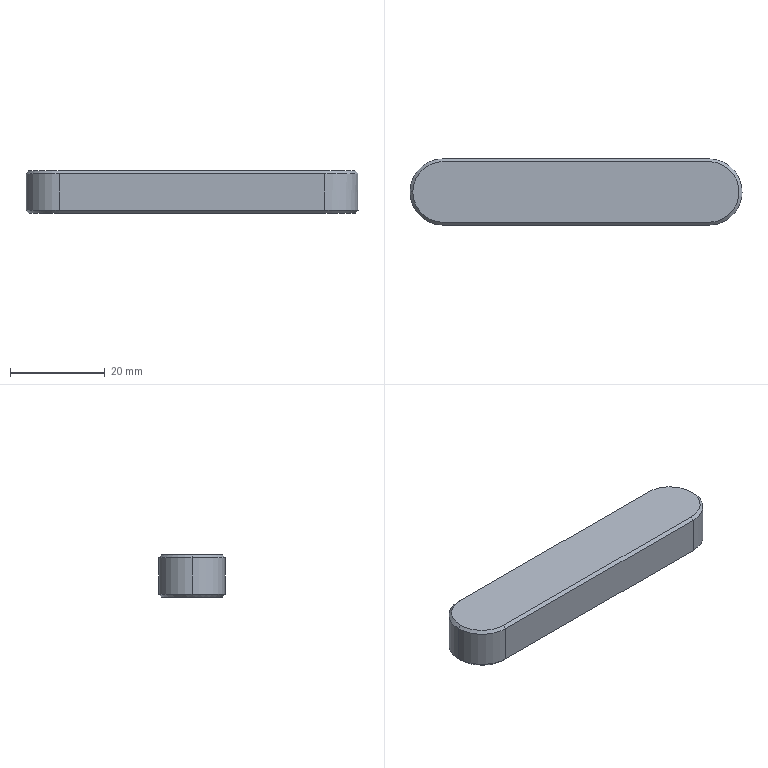Part | SolidWorks | features Boss 2, Chamfer 1, Extrusion 1 | 1 solid | 17 faces | box 70 x 14 x 9 mm | volume 8386 mm3 | plane 8 | cone 6 | cylinder 3 | commonest cylinder face diameters 14 x3
STEP:
#1=CARTESIAN_POINT('',(-62.4,0.,4.5));
#2=VERTEX_POINT('',#1);
#3=CARTESIAN_POINT('',(-56.,-6.4,4.5));
#4=VERTEX_POINT('',#3);
#5=CARTESIAN_POINT('',(-56.,0.,4.5));
#6=DIRECTION('',(0.,0.,1.));
#7=DIRECTION('',(-1.,0.,0.));
#8=AXIS2_PLACEMENT_3D('',#5,#6,#7);
#9=CIRCLE('',#8,6.4);
#10=EDGE_CURVE('',#2,#4,#9,.T.);
#11=ORIENTED_EDGE('',*,*,#10,.F.);
#12=CARTESIAN_POINT('',(-63.,0.,3.9));
#13=VERTEX_POINT('',#12);
#14=CARTESIAN_POINT('',(-62.4,0.,4.5));
#15=DIRECTION('',(-0.7071,0.,-0.7071));
#16=VECTOR('',#15,1000.);
#17=LINE('',#14,#16);
#18=EDGE_CURVE('',#2,#13,#17,.T.);
#19=ORIENTED_EDGE('',*,*,#18,.T.);
#20=CARTESIAN_POINT('',(-56.,-7.,3.9));
#21=VERTEX_POINT('',#20);
#22=CARTESIAN_POINT('',(-56.,0.,3.9));
#23=DIRECTION('',(0.,0.,-1.));
#24=DIRECTION('',(-1.,0.,0.));
#25=AXIS2_PLACEMENT_3D('',#22,#23,#24);
#26=CIRCLE('',#25,7.);
#27=EDGE_CURVE('',#21,#13,#26,.T.);
#28=ORIENTED_EDGE('',*,*,#27,.F.);
#29=CARTESIAN_POINT('',(-56.,-6.4,4.5));
#30=DIRECTION('',(0.,-0.7071,-0.7071));
#31=VECTOR('',#30,1000.);
#32=LINE('',#29,#31);
#33=EDGE_CURVE('',#4,#21,#32,.T.);
#34=ORIENTED_EDGE('',*,*,#33,.F.);
#35=EDGE_LOOP('',(#11,#19,#28,#34));
#36=FACE_OUTER_BOUND('',#35,.T.);
#37=CARTESIAN_POINT('',(-56.,0.,4.5));
#38=DIRECTION('',(0.,0.,-1.));
#39=DIRECTION('',(-1.,0.,0.));
#40=AXIS2_PLACEMENT_3D('',#37,#38,#39);
#41=CONICAL_SURFACE('',#40,6.4,0.7854);
#42=ADVANCED_FACE('',(#36),#41,.T.);
#43=CARTESIAN_POINT('',(6.4,0.,-4.5));
#44=VERTEX_POINT('',#43);
#45=CARTESIAN_POINT('',(0.,-6.4,-4.5));
#46=VERTEX_POINT('',#45);
#47=CARTESIAN_POINT('',(0.,0.,-4.5));
#48=DIRECTION('',(0.,0.,-1.));
#49=DIRECTION('',(-1.,0.,0.));
#50=AXIS2_PLACEMENT_3D('',#47,#48,#49);
#51=CIRCLE('',#50,6.4);
#52=EDGE_CURVE('',#44,#46,#51,.T.);
#53=ORIENTED_EDGE('',*,*,#52,.F.);
#54=CARTESIAN_POINT('',(7.,0.,-3.9));
#55=VERTEX_POINT('',#54);
#56=CARTESIAN_POINT('',(7.,0.,-3.9));
#57=DIRECTION('',(0.7071,0.,0.7071));
#58=VECTOR('',#57,1000.);
#59=LINE('',#56,#58);
#60=EDGE_CURVE('',#44,#55,#59,.T.);
#61=ORIENTED_EDGE('',*,*,#60,.T.);
#62=CARTESIAN_POINT('',(0.,-7.,-3.9));
#63=VERTEX_POINT('',#62);
#64=CARTESIAN_POINT('',(0.,0.,-3.9));
#65=DIRECTION('',(0.,0.,1.));
#66=DIRECTION('',(-1.,0.,0.));
#67=AXIS2_PLACEMENT_3D('',#64,#65,#66);
#68=CIRCLE('',#67,7.);
#69=EDGE_CURVE('',#63,#55,#68,.T.);
#70=ORIENTED_EDGE('',*,*,#69,.F.);
#71=CARTESIAN_POINT('',(0.,-6.4,-4.5));
#72=DIRECTION('',(0.,-0.7071,0.7071));
#73=VECTOR('',#72,1000.);
#74=LINE('',#71,#73);
#75=EDGE_CURVE('',#46,#63,#74,.T.);
#76=ORIENTED_EDGE('',*,*,#75,.F.);
#77=EDGE_LOOP('',(#53,#61,#70,#76));
#78=FACE_OUTER_BOUND('',#77,.T.);
#79=CARTESIAN_POINT('',(0.,0.,-3.9));
#80=DIRECTION('',(0.,0.,1.));
#81=DIRECTION('',(1.,0.,0.));
#82=AXIS2_PLACEMENT_3D('',#79,#80,#81);
#83=CONICAL_SURFACE('',#82,7.,0.7854);
#84=ADVANCED_FACE('',(#78),#83,.T.);
#85=ORIENTED_EDGE('',*,*,#27,.T.);
#86=CARTESIAN_POINT('',(-63.,0.,-3.9));
#87=VERTEX_POINT('',#86);
#88=CARTESIAN_POINT('',(-63.,0.,4.5));
#89=DIRECTION('',(0.,0.,-1.));
#90=VECTOR('',#89,1000.);
#91=LINE('',#88,#90);
#92=EDGE_CURVE('',#13,#87,#91,.T.);
#93=ORIENTED_EDGE('',*,*,#92,.T.);
#94=CARTESIAN_POINT('',(-56.,-7.,-3.9));
#95=VERTEX_POINT('',#94);
#96=CARTESIAN_POINT('',(-56.,0.,-3.9));
#97=DIRECTION('',(0.,0.,1.));
#98=DIRECTION('',(-1.,0.,0.));
#99=AXIS2_PLACEMENT_3D('',#96,#97,#98);
#100=CIRCLE('',#99,7.);
#101=EDGE_CURVE('',#87,#95,#100,.T.);
#102=ORIENTED_EDGE('',*,*,#101,.T.);
#103=CARTESIAN_POINT('',(-56.,-7.,4.5));
#104=DIRECTION('',(0.,0.,-1.));
#105=VECTOR('',#104,1000.);
#106=LINE('',#103,#105);
#107=EDGE_CURVE('',#21,#95,#106,.T.);
#108=ORIENTED_EDGE('',*,*,#107,.F.);
#109=EDGE_LOOP('',(#85,#93,#102,#108));
#110=FACE_OUTER_BOUND('',#109,.T.);
#111=CARTESIAN_POINT('',(-56.,0.,4.5));
#112=DIRECTION('',(0.,0.,-1.));
#113=DIRECTION('',(-1.,0.,0.));
#114=AXIS2_PLACEMENT_3D('',#111,#112,#113);
#115=CYLINDRICAL_SURFACE('',#114,7.);
#116=ADVANCED_FACE('',(#110),#115,.T.);
#117=ORIENTED_EDGE('',*,*,#92,.F.);
#118=CARTESIAN_POINT('',(-56.,7.,3.9));
#119=VERTEX_POINT('',#118);
#120=CARTESIAN_POINT('',(-56.,0.,3.9));
#121=DIRECTION('',(0.,0.,-1.));
#122=DIRECTION('',(-1.,0.,0.));
#123=AXIS2_PLACEMENT_3D('',#120,#121,#122);
#124=CIRCLE('',#123,7.);
#125=EDGE_CURVE('',#13,#119,#124,.T.);
#126=ORIENTED_EDGE('',*,*,#125,.T.);
#127=CARTESIAN_POINT('',(-56.,7.,-3.9));
#128=VERTEX_POINT('',#127);
#129=CARTESIAN_POINT('',(-56.,7.,4.5));
#130=DIRECTION('',(0.,0.,-1.));
#131=VECTOR('',#130,1000.);
#132=LINE('',#129,#131);
#133=EDGE_CURVE('',#119,#128,#132,.T.);
#134=ORIENTED_EDGE('',*,*,#133,.T.);
#135=CARTESIAN_POINT('',(-56.,0.,-3.9));
#136=DIRECTION('',(0.,0.,1.));
#137=DIRECTION('',(-1.,0.,0.));
#138=AXIS2_PLACEMENT_3D('',#135,#136,#137);
#139=CIRCLE('',#138,7.);
#140=EDGE_CURVE('',#128,#87,#139,.T.);
#141=ORIENTED_EDGE('',*,*,#140,.T.);
#142=EDGE_LOOP('',(#117,#126,#134,#141));
#143=FACE_OUTER_BOUND('',#142,.T.);
#144=CARTESIAN_POINT('',(-56.,0.,4.5));
#145=DIRECTION('',(0.,0.,-1.));
#146=DIRECTION('',(-1.,0.,0.));
#147=AXIS2_PLACEMENT_3D('',#144,#145,#146);
#148=CYLINDRICAL_SURFACE('',#147,7.);
#149=ADVANCED_FACE('',(#143),#148,.T.);
#150=ORIENTED_EDGE('',*,*,#107,.T.);
#151=CARTESIAN_POINT('',(0.,-7.,-3.9));
#152=DIRECTION('',(1.,0.,0.));
#153=VECTOR('',#152,1000.);
#154=LINE('',#151,#153);
#155=EDGE_CURVE('',#95,#63,#154,.T.);
#156=ORIENTED_EDGE('',*,*,#155,.T.);
#157=CARTESIAN_POINT('',(0.,-7.,3.9));
#158=VERTEX_POINT('',#157);
#159=CARTESIAN_POINT('',(0.,-7.,4.5));
#160=DIRECTION('',(0.,0.,-1.));
#161=VECTOR('',#160,1000.);
#162=LINE('',#159,#161);
#163=EDGE_CURVE('',#158,#63,#162,.T.);
#164=ORIENTED_EDGE('',*,*,#163,.F.);
#165=CARTESIAN_POINT('',(0.,-7.,3.9));
#166=DIRECTION('',(-1.,0.,0.));
#167=VECTOR('',#166,1000.);
#168=LINE('',#165,#167);
#169=EDGE_CURVE('',#158,#21,#168,.T.);
#170=ORIENTED_EDGE('',*,*,#169,.T.);
#171=EDGE_LOOP('',(#150,#156,#164,#170));
#172=FACE_OUTER_BOUND('',#171,.T.);
#173=CARTESIAN_POINT('',(0.,-7.,4.5));
#174=DIRECTION('',(0.,1.,0.));
#175=DIRECTION('',(-1.,0.,0.));
#176=AXIS2_PLACEMENT_3D('',#173,#174,#175);
#177=PLANE('',#176);
#178=ADVANCED_FACE('',(#172),#177,.F.);
#179=CARTESIAN_POINT('',(0.,7.,3.9));
#180=VERTEX_POINT('',#179);
#181=CARTESIAN_POINT('',(0.,7.,-3.9));
#182=VERTEX_POINT('',#181);
#183=CARTESIAN_POINT('',(0.,7.,4.5));
#184=DIRECTION('',(0.,0.,-1.));
#185=VECTOR('',#184,1000.);
#186=LINE('',#183,#185);
#187=EDGE_CURVE('',#180,#182,#186,.T.);
#188=ORIENTED_EDGE('',*,*,#187,.F.);
#189=CARTESIAN_POINT('',(0.,0.,3.9));
#190=DIRECTION('',(0.,0.,-1.));
#191=DIRECTION('',(-1.,0.,0.));
#192=AXIS2_PLACEMENT_3D('',#189,#190,#191);
#193=CIRCLE('',#192,7.);
#194=EDGE_CURVE('',#180,#158,#193,.T.);
#195=ORIENTED_EDGE('',*,*,#194,.T.);
#196=ORIENTED_EDGE('',*,*,#163,.T.);
#197=ORIENTED_EDGE('',*,*,#69,.T.);
#198=CARTESIAN_POINT('',(0.,0.,-3.9));
#199=DIRECTION('',(0.,0.,1.));
#200=DIRECTION('',(-1.,0.,0.));
#201=AXIS2_PLACEMENT_3D('',#198,#199,#200);
#202=CIRCLE('',#201,7.);
#203=EDGE_CURVE('',#55,#182,#202,.T.);
#204=ORIENTED_EDGE('',*,*,#203,.T.);
#205=EDGE_LOOP('',(#188,#195,#196,#197,#204));
#206=FACE_OUTER_BOUND('',#205,.T.);
#207=CARTESIAN_POINT('',(0.,0.,4.5));
#208=DIRECTION('',(0.,0.,-1.));
#209=DIRECTION('',(-1.,0.,0.));
#210=AXIS2_PLACEMENT_3D('',#207,#208,#209);
#211=CYLINDRICAL_SURFACE('',#210,7.);
#212=ADVANCED_FACE('',(#206),#211,.T.);
#213=ORIENTED_EDGE('',*,*,#133,.F.);
#214=CARTESIAN_POINT('',(-56.,7.,3.9));
#215=DIRECTION('',(1.,0.,0.));
#216=VECTOR('',#215,1000.);
#217=LINE('',#214,#216);
#218=EDGE_CURVE('',#119,#180,#217,.T.);
#219=ORIENTED_EDGE('',*,*,#218,.T.);
#220=ORIENTED_EDGE('',*,*,#187,.T.);
#221=CARTESIAN_POINT('',(-56.,7.,-3.9));
#222=DIRECTION('',(-1.,0.,0.));
#223=VECTOR('',#222,1000.);
#224=LINE('',#221,#223);
#225=EDGE_CURVE('',#182,#128,#224,.T.);
#226=ORIENTED_EDGE('',*,*,#225,.T.);
#227=EDGE_LOOP('',(#213,#219,#220,#226));
#228=FACE_OUTER_BOUND('',#227,.T.);
#229=CARTESIAN_POINT('',(-56.,7.,4.5));
#230=DIRECTION('',(0.,-1.,0.));
#231=DIRECTION('',(1.,0.,0.));
#232=AXIS2_PLACEMENT_3D('',#229,#230,#231);
#233=PLANE('',#232);
#234=ADVANCED_FACE('',(#228),#233,.F.);
#235=CARTESIAN_POINT('',(-56.,6.4,4.5));
#236=VERTEX_POINT('',#235);
#237=CARTESIAN_POINT('',(-56.,0.,4.5));
#238=DIRECTION('',(0.,0.,1.));
#239=DIRECTION('',(-1.,0.,0.));
#240=AXIS2_PLACEMENT_3D('',#237,#238,#239);
#241=CIRCLE('',#240,6.4);
#242=EDGE_CURVE('',#236,#2,#241,.T.);
#243=ORIENTED_EDGE('',*,*,#242,.T.);
#244=ORIENTED_EDGE('',*,*,#10,.T.);
#245=CARTESIAN_POINT('',(0.,-6.4,4.5));
#246=VERTEX_POINT('',#245);
#247=CARTESIAN_POINT('',(-56.,-6.4,4.5));
#248=DIRECTION('',(1.,0.,0.));
#249=VECTOR('',#248,1000.);
#250=LINE('',#247,#249);
#251=EDGE_CURVE('',#4,#246,#250,.T.);
#252=ORIENTED_EDGE('',*,*,#251,.T.);
#253=CARTESIAN_POINT('',(0.,6.4,4.5));
#254=VERTEX_POINT('',#253);
#255=CARTESIAN_POINT('',(0.,0.,4.5));
#256=DIRECTION('',(0.,0.,1.));
#257=DIRECTION('',(-1.,0.,0.));
#258=AXIS2_PLACEMENT_3D('',#255,#256,#257);
#259=CIRCLE('',#258,6.4);
#260=EDGE_CURVE('',#246,#254,#259,.T.);
#261=ORIENTED_EDGE('',*,*,#260,.T.);
#262=CARTESIAN_POINT('',(-56.,6.4,4.5));
#263=DIRECTION('',(-1.,0.,0.));
#264=VECTOR('',#263,1000.);
#265=LINE('',#262,#264);
#266=EDGE_CURVE('',#254,#236,#265,.T.);
#267=ORIENTED_EDGE('',*,*,#266,.T.);
#268=EDGE_LOOP('',(#243,#244,#252,#261,#267));
#269=FACE_OUTER_BOUND('',#268,.T.);
#270=CARTESIAN_POINT('',(-56.,0.,4.5));
#271=DIRECTION('',(0.,0.,-1.));
#272=DIRECTION('',(-1.,0.,0.));
#273=AXIS2_PLACEMENT_3D('',#270,#271,#272);
#274=PLANE('',#273);
#275=ADVANCED_FACE('',(#269),#274,.F.);
#276=CARTESIAN_POINT('',(0.,6.4,-4.5));
#277=VERTEX_POINT('',#276);
#278=CARTESIAN_POINT('',(0.,0.,-4.5));
#279=DIRECTION('',(0.,0.,-1.));
#280=DIRECTION('',(-1.,0.,0.));
#281=AXIS2_PLACEMENT_3D('',#278,#279,#280);
#282=CIRCLE('',#281,6.4);
#283=EDGE_CURVE('',#277,#44,#282,.T.);
#284=ORIENTED_EDGE('',*,*,#283,.T.);
#285=ORIENTED_EDGE('',*,*,#52,.T.);
#286=CARTESIAN_POINT('',(-56.,-6.4,-4.5));
#287=VERTEX_POINT('',#286);
#288=CARTESIAN_POINT('',(-56.,-6.4,-4.5));
#289=DIRECTION('',(-1.,0.,0.));
#290=VECTOR('',#289,1000.);
#291=LINE('',#288,#290);
#292=EDGE_CURVE('',#46,#287,#291,.T.);
#293=ORIENTED_EDGE('',*,*,#292,.T.);
#294=CARTESIAN_POINT('',(-56.,6.4,-4.5));
#295=VERTEX_POINT('',#294);
#296=CARTESIAN_POINT('',(-56.,0.,-4.5));
#297=DIRECTION('',(0.,0.,-1.));
#298=DIRECTION('',(-1.,0.,0.));
#299=AXIS2_PLACEMENT_3D('',#296,#297,#298);
#300=CIRCLE('',#299,6.4);
#301=EDGE_CURVE('',#287,#295,#300,.T.);
#302=ORIENTED_EDGE('',*,*,#301,.T.);
#303=CARTESIAN_POINT('',(0.,6.4,-4.5));
#304=DIRECTION('',(1.,0.,0.));
#305=VECTOR('',#304,1000.);
#306=LINE('',#303,#305);
#307=EDGE_CURVE('',#295,#277,#306,.T.);
#308=ORIENTED_EDGE('',*,*,#307,.T.);
#309=EDGE_LOOP('',(#284,#285,#293,#302,#308));
#310=FACE_OUTER_BOUND('',#309,.T.);
#311=CARTESIAN_POINT('',(-56.,0.,-4.5));
#312=DIRECTION('',(0.,0.,-1.));
#313=DIRECTION('',(-1.,0.,0.));
#314=AXIS2_PLACEMENT_3D('',#311,#312,#313);
#315=PLANE('',#314);
#316=ADVANCED_FACE('',(#310),#315,.T.);
#317=CARTESIAN_POINT('',(0.,6.4,-4.5));
#318=DIRECTION('',(0.,0.7071,0.7071));
#319=VECTOR('',#318,1000.);
#320=LINE('',#317,#319);
#321=EDGE_CURVE('',#277,#182,#320,.T.);
#322=ORIENTED_EDGE('',*,*,#321,.F.);
#323=ORIENTED_EDGE('',*,*,#307,.F.);
#324=CARTESIAN_POINT('',(-56.,7.,-3.9));
#325=DIRECTION('',(0.,-0.7071,-0.7071));
#326=VECTOR('',#325,1000.);
#327=LINE('',#324,#326);
#328=EDGE_CURVE('',#128,#295,#327,.T.);
#329=ORIENTED_EDGE('',*,*,#328,.F.);
#330=ORIENTED_EDGE('',*,*,#225,.F.);
#331=EDGE_LOOP('',(#322,#323,#329,#330));
#332=FACE_OUTER_BOUND('',#331,.T.);
#333=CARTESIAN_POINT('',(-56.,7.,-3.9));
#334=DIRECTION('',(0.,0.7071,-0.7071));
#335=DIRECTION('',(0.,0.7071,0.7071));
#336=AXIS2_PLACEMENT_3D('',#333,#334,#335);
#337=PLANE('',#336);
#338=ADVANCED_FACE('',(#332),#337,.T.);
#339=ORIENTED_EDGE('',*,*,#328,.T.);
#340=ORIENTED_EDGE('',*,*,#301,.F.);
#341=CARTESIAN_POINT('',(-56.,-7.,-3.9));
#342=DIRECTION('',(0.,0.7071,-0.7071));
#343=VECTOR('',#342,1000.);
#344=LINE('',#341,#343);
#345=EDGE_CURVE('',#95,#287,#344,.T.);
#346=ORIENTED_EDGE('',*,*,#345,.F.);
#347=ORIENTED_EDGE('',*,*,#101,.F.);
#348=ORIENTED_EDGE('',*,*,#140,.F.);
#349=EDGE_LOOP('',(#339,#340,#346,#347,#348));
#350=FACE_OUTER_BOUND('',#349,.T.);
#351=CARTESIAN_POINT('',(-56.,0.,-3.9));
#352=DIRECTION('',(0.,0.,1.));
#353=DIRECTION('',(1.,0.,0.));
#354=AXIS2_PLACEMENT_3D('',#351,#352,#353);
#355=CONICAL_SURFACE('',#354,7.,0.7854);
#356=ADVANCED_FACE('',(#350),#355,.T.);
#357=ORIENTED_EDGE('',*,*,#60,.F.);
#358=ORIENTED_EDGE('',*,*,#283,.F.);
#359=ORIENTED_EDGE('',*,*,#321,.T.);
#360=ORIENTED_EDGE('',*,*,#203,.F.);
#361=EDGE_LOOP('',(#357,#358,#359,#360));
#362=FACE_OUTER_BOUND('',#361,.T.);
#363=CARTESIAN_POINT('',(0.,0.,-3.9));
#364=DIRECTION('',(0.,0.,1.));
#365=DIRECTION('',(1.,0.,0.));
#366=AXIS2_PLACEMENT_3D('',#363,#364,#365);
#367=CONICAL_SURFACE('',#366,7.,0.7854);
#368=ADVANCED_FACE('',(#362),#367,.T.);
#369=ORIENTED_EDGE('',*,*,#345,.T.);
#370=ORIENTED_EDGE('',*,*,#292,.F.);
#371=ORIENTED_EDGE('',*,*,#75,.T.);
#372=ORIENTED_EDGE('',*,*,#155,.F.);
#373=EDGE_LOOP('',(#369,#370,#371,#372));
#374=FACE_OUTER_BOUND('',#373,.T.);
#375=CARTESIAN_POINT('',(0.,-7.,-3.9));
#376=DIRECTION('',(0.,-0.7071,-0.7071));
#377=DIRECTION('',(0.,0.7071,-0.7071));
#378=AXIS2_PLACEMENT_3D('',#375,#376,#377);
#379=PLANE('',#378);
#380=ADVANCED_FACE('',(#374),#379,.T.);
#381=CARTESIAN_POINT('',(0.,7.,3.9));
#382=DIRECTION('',(0.,-0.7071,0.7071));
#383=VECTOR('',#382,1000.);
#384=LINE('',#381,#383);
#385=EDGE_CURVE('',#180,#254,#384,.T.);
#386=ORIENTED_EDGE('',*,*,#385,.F.);
#387=ORIENTED_EDGE('',*,*,#218,.F.);
#388=CARTESIAN_POINT('',(-56.,6.4,4.5));
#389=DIRECTION('',(0.,0.7071,-0.7071));
#390=VECTOR('',#389,1000.);
#391=LINE('',#388,#390);
#392=EDGE_CURVE('',#236,#119,#391,.T.);
#393=ORIENTED_EDGE('',*,*,#392,.F.);
#394=ORIENTED_EDGE('',*,*,#266,.F.);
#395=EDGE_LOOP('',(#386,#387,#393,#394));
#396=FACE_OUTER_BOUND('',#395,.T.);
#397=CARTESIAN_POINT('',(-56.,6.4,4.5));
#398=DIRECTION('',(0.,-0.7071,-0.7071));
#399=DIRECTION('',(0.,0.7071,-0.7071));
#400=AXIS2_PLACEMENT_3D('',#397,#398,#399);
#401=PLANE('',#400);
#402=ADVANCED_FACE('',(#396),#401,.F.);
#403=ORIENTED_EDGE('',*,*,#18,.F.);
#404=ORIENTED_EDGE('',*,*,#242,.F.);
#405=ORIENTED_EDGE('',*,*,#392,.T.);
#406=ORIENTED_EDGE('',*,*,#125,.F.);
#407=EDGE_LOOP('',(#403,#404,#405,#406));
#408=FACE_OUTER_BOUND('',#407,.T.);
#409=CARTESIAN_POINT('',(-56.,0.,4.5));
#410=DIRECTION('',(0.,0.,-1.));
#411=DIRECTION('',(-1.,0.,0.));
#412=AXIS2_PLACEMENT_3D('',#409,#410,#411);
#413=CONICAL_SURFACE('',#412,6.4,0.7854);
#414=ADVANCED_FACE('',(#408),#413,.T.);
#415=ORIENTED_EDGE('',*,*,#385,.T.);
#416=ORIENTED_EDGE('',*,*,#260,.F.);
#417=CARTESIAN_POINT('',(0.,-7.,3.9));
#418=DIRECTION('',(0.,0.7071,0.7071));
#419=VECTOR('',#418,1000.);
#420=LINE('',#417,#419);
#421=EDGE_CURVE('',#158,#246,#420,.T.);
#422=ORIENTED_EDGE('',*,*,#421,.F.);
#423=ORIENTED_EDGE('',*,*,#194,.F.);
#424=EDGE_LOOP('',(#415,#416,#422,#423));
#425=FACE_OUTER_BOUND('',#424,.T.);
#426=CARTESIAN_POINT('',(0.,0.,4.5));
#427=DIRECTION('',(0.,0.,-1.));
#428=DIRECTION('',(-1.,0.,0.));
#429=AXIS2_PLACEMENT_3D('',#426,#427,#428);
#430=CONICAL_SURFACE('',#429,6.4,0.7854);
#431=ADVANCED_FACE('',(#425),#430,.T.);
#432=ORIENTED_EDGE('',*,*,#33,.T.);
#433=ORIENTED_EDGE('',*,*,#169,.F.);
#434=ORIENTED_EDGE('',*,*,#421,.T.);
#435=ORIENTED_EDGE('',*,*,#251,.F.);
#436=EDGE_LOOP('',(#432,#433,#434,#435));
#437=FACE_OUTER_BOUND('',#436,.T.);
#438=CARTESIAN_POINT('',(-56.,-6.4,4.5));
#439=DIRECTION('',(0.,0.7071,-0.7071));
#440=DIRECTION('',(0.,0.7071,0.7071));
#441=AXIS2_PLACEMENT_3D('',#438,#439,#440);
#442=PLANE('',#441);
#443=ADVANCED_FACE('',(#437),#442,.F.);
#444=CLOSED_SHELL('',(#42,#84,#116,#149,#178,#212,#234,#275,#316,#338,#356,#368,#380,#402,#414,#431,#443));
#445=MANIFOLD_SOLID_BREP('',#444);
#446=CARTESIAN_POINT('',(0.,0.,0.));
#447=DIRECTION('',(0.,0.,1.));
#448=DIRECTION('',(1.,0.,0.));
#449=AXIS2_PLACEMENT_3D('',#446,#447,#448);
#450=(LENGTH_UNIT()NAMED_UNIT(*)SI_UNIT(.MILLI.,.METRE.));
#451=UNCERTAINTY_MEASURE_WITH_UNIT(LENGTH_MEASURE(0.00001),#450,'','');
#452=(NAMED_UNIT(*)PLANE_ANGLE_UNIT()SI_UNIT($,.RADIAN.));
#453=(NAMED_UNIT(*)SI_UNIT($,.STERADIAN.)SOLID_ANGLE_UNIT());
#454=(GEOMETRIC_REPRESENTATION_CONTEXT(3)GLOBAL_UNCERTAINTY_ASSIGNED_CONTEXT((#451))GLOBAL_UNIT_ASSIGNED_CONTEXT((#450,#452,#453))REPRESENTATION_CONTEXT('',''));
#455=ADVANCED_BREP_SHAPE_REPRESENTATION('',(#445,#449),#454);